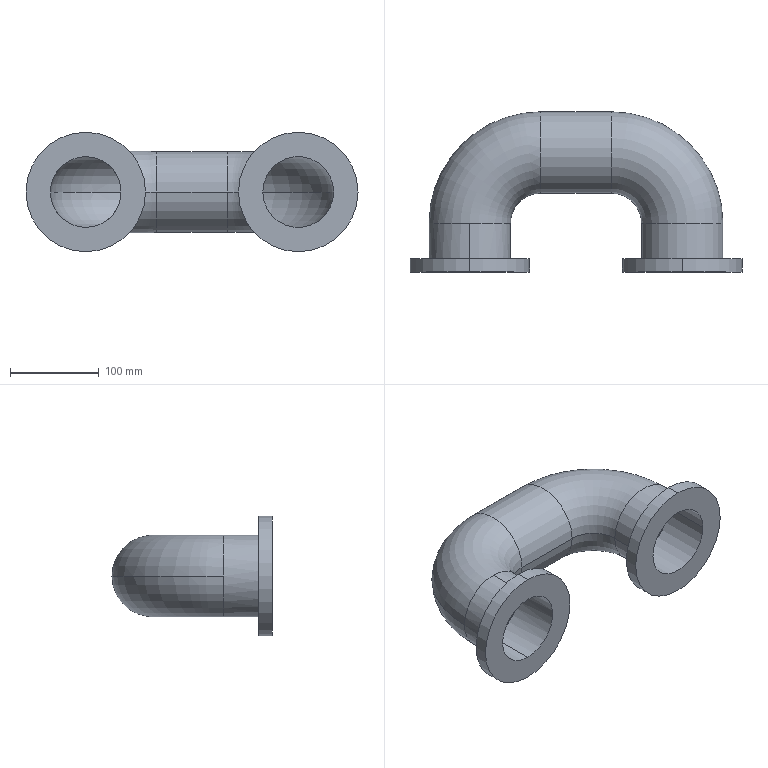Part | SolidWorks | features ICE 1, Sweep 1 | 1 solid | 28 faces | box 375 x 181 x 135 mm | volume 945407 mm3 | cylinder 16 | torus 8 | plane 4 | commonest cylinder face diameters 80 x6 92 x6 135 x4
STEP:
#1=CARTESIAN_POINT('',(160.,80.,0.));
#2=VERTEX_POINT('',#1);
#3=CARTESIAN_POINT('',(160.,160.,0.));
#4=VERTEX_POINT('',#3);
#5=CARTESIAN_POINT('',(160.,120.,0.));
#6=DIRECTION('',(-1.,0.,0.));
#7=DIRECTION('',(0.,0.,1.));
#8=AXIS2_PLACEMENT_3D('',#5,#6,#7);
#9=CIRCLE('',#8,40.);
#10=EDGE_CURVE('',#2,#4,#9,.T.);
#11=ORIENTED_EDGE('',*,*,#10,.T.);
#12=CARTESIAN_POINT('',(280.,40.,0.));
#13=VERTEX_POINT('',#12);
#14=CARTESIAN_POINT('',(160.,40.,0.));
#15=DIRECTION('',(0.,0.,-1.));
#16=DIRECTION('',(-1.,0.,0.));
#17=AXIS2_PLACEMENT_3D('',#14,#15,#16);
#18=CIRCLE('',#17,120.);
#19=EDGE_CURVE('',#4,#13,#18,.T.);
#20=ORIENTED_EDGE('',*,*,#19,.T.);
#21=CARTESIAN_POINT('',(200.,40.,0.));
#22=VERTEX_POINT('',#21);
#23=CARTESIAN_POINT('',(240.,40.,0.));
#24=DIRECTION('',(0.,1.,0.));
#25=DIRECTION('',(0.,0.,1.));
#26=AXIS2_PLACEMENT_3D('',#23,#24,#25);
#27=CIRCLE('',#26,40.);
#28=EDGE_CURVE('',#22,#13,#27,.T.);
#29=ORIENTED_EDGE('',*,*,#28,.F.);
#30=CARTESIAN_POINT('',(160.,40.,0.));
#31=DIRECTION('',(0.,0.,-1.));
#32=DIRECTION('',(-1.,0.,0.));
#33=AXIS2_PLACEMENT_3D('',#30,#31,#32);
#34=CIRCLE('',#33,40.);
#35=EDGE_CURVE('',#2,#22,#34,.T.);
#36=ORIENTED_EDGE('',*,*,#35,.F.);
#37=EDGE_LOOP('',(#11,#20,#29,#36));
#38=FACE_OUTER_BOUND('',#37,.T.);
#39=CARTESIAN_POINT('',(160.,40.,0.));
#40=DIRECTION('',(0.,0.,-1.));
#41=DIRECTION('',(-1.,0.,0.));
#42=AXIS2_PLACEMENT_3D('',#39,#40,#41);
#43=TOROIDAL_SURFACE('',#42,80.,40.);
#44=ADVANCED_FACE('',(#38),#43,.F.);
#45=CARTESIAN_POINT('',(0.,40.,40.));
#46=VERTEX_POINT('',#45);
#47=CARTESIAN_POINT('',(-40.,40.,0.));
#48=VERTEX_POINT('',#47);
#49=CARTESIAN_POINT('',(0.,40.,0.));
#50=DIRECTION('',(0.,-1.,0.));
#51=DIRECTION('',(0.,0.,1.));
#52=AXIS2_PLACEMENT_3D('',#49,#50,#51);
#53=CIRCLE('',#52,40.);
#54=EDGE_CURVE('',#46,#48,#53,.T.);
#55=ORIENTED_EDGE('',*,*,#54,.T.);
#56=CARTESIAN_POINT('',(80.,160.,0.));
#57=VERTEX_POINT('',#56);
#58=CARTESIAN_POINT('',(80.,40.,0.));
#59=DIRECTION('',(0.,0.,-1.));
#60=DIRECTION('',(-1.,0.,0.));
#61=AXIS2_PLACEMENT_3D('',#58,#59,#60);
#62=CIRCLE('',#61,120.);
#63=EDGE_CURVE('',#48,#57,#62,.T.);
#64=ORIENTED_EDGE('',*,*,#63,.T.);
#65=CARTESIAN_POINT('',(80.,80.,0.));
#66=VERTEX_POINT('',#65);
#67=CARTESIAN_POINT('',(80.,120.,0.));
#68=DIRECTION('',(-1.,0.,0.));
#69=DIRECTION('',(0.,0.,1.));
#70=AXIS2_PLACEMENT_3D('',#67,#68,#69);
#71=CIRCLE('',#70,40.);
#72=EDGE_CURVE('',#66,#57,#71,.T.);
#73=ORIENTED_EDGE('',*,*,#72,.F.);
#74=CARTESIAN_POINT('',(40.,40.,0.));
#75=VERTEX_POINT('',#74);
#76=CARTESIAN_POINT('',(80.,40.,0.));
#77=DIRECTION('',(0.,0.,-1.));
#78=DIRECTION('',(-1.,0.,0.));
#79=AXIS2_PLACEMENT_3D('',#76,#77,#78);
#80=CIRCLE('',#79,40.);
#81=EDGE_CURVE('',#75,#66,#80,.T.);
#82=ORIENTED_EDGE('',*,*,#81,.F.);
#83=CARTESIAN_POINT('',(0.,40.,0.));
#84=DIRECTION('',(0.,-1.,0.));
#85=DIRECTION('',(0.,0.,1.));
#86=AXIS2_PLACEMENT_3D('',#83,#84,#85);
#87=CIRCLE('',#86,40.);
#88=EDGE_CURVE('',#75,#46,#87,.T.);
#89=ORIENTED_EDGE('',*,*,#88,.T.);
#90=EDGE_LOOP('',(#55,#64,#73,#82,#89));
#91=FACE_OUTER_BOUND('',#90,.T.);
#92=CARTESIAN_POINT('',(80.,40.,0.));
#93=DIRECTION('',(0.,0.,-1.));
#94=DIRECTION('',(-1.,0.,0.));
#95=AXIS2_PLACEMENT_3D('',#92,#93,#94);
#96=TOROIDAL_SURFACE('',#95,80.,40.);
#97=ADVANCED_FACE('',(#91),#96,.F.);
#98=CARTESIAN_POINT('',(160.,74.,0.));
#99=VERTEX_POINT('',#98);
#100=CARTESIAN_POINT('',(160.,166.,0.));
#101=VERTEX_POINT('',#100);
#102=CARTESIAN_POINT('',(160.,120.,0.));
#103=DIRECTION('',(1.,0.,0.));
#104=DIRECTION('',(0.,0.,1.));
#105=AXIS2_PLACEMENT_3D('',#102,#103,#104);
#106=CIRCLE('',#105,46.);
#107=EDGE_CURVE('',#99,#101,#106,.T.);
#108=ORIENTED_EDGE('',*,*,#107,.T.);
#109=CARTESIAN_POINT('',(286.,40.,0.));
#110=VERTEX_POINT('',#109);
#111=CARTESIAN_POINT('',(160.,40.,0.));
#112=DIRECTION('',(0.,0.,-1.));
#113=DIRECTION('',(-1.,0.,0.));
#114=AXIS2_PLACEMENT_3D('',#111,#112,#113);
#115=CIRCLE('',#114,126.);
#116=EDGE_CURVE('',#101,#110,#115,.T.);
#117=ORIENTED_EDGE('',*,*,#116,.T.);
#118=CARTESIAN_POINT('',(194.,40.,0.));
#119=VERTEX_POINT('',#118);
#120=CARTESIAN_POINT('',(240.,40.,0.));
#121=DIRECTION('',(0.,-1.,0.));
#122=DIRECTION('',(0.,0.,1.));
#123=AXIS2_PLACEMENT_3D('',#120,#121,#122);
#124=CIRCLE('',#123,46.);
#125=EDGE_CURVE('',#119,#110,#124,.T.);
#126=ORIENTED_EDGE('',*,*,#125,.F.);
#127=CARTESIAN_POINT('',(160.,40.,0.));
#128=DIRECTION('',(0.,0.,-1.));
#129=DIRECTION('',(-1.,0.,0.));
#130=AXIS2_PLACEMENT_3D('',#127,#128,#129);
#131=CIRCLE('',#130,34.);
#132=EDGE_CURVE('',#99,#119,#131,.T.);
#133=ORIENTED_EDGE('',*,*,#132,.F.);
#134=EDGE_LOOP('',(#108,#117,#126,#133));
#135=FACE_OUTER_BOUND('',#134,.T.);
#136=CARTESIAN_POINT('',(160.,40.,0.));
#137=DIRECTION('',(0.,0.,-1.));
#138=DIRECTION('',(-1.,0.,0.));
#139=AXIS2_PLACEMENT_3D('',#136,#137,#138);
#140=TOROIDAL_SURFACE('',#139,80.,46.);
#141=ADVANCED_FACE('',(#135),#140,.T.);
#142=CARTESIAN_POINT('',(0.,40.,-46.));
#143=VERTEX_POINT('',#142);
#144=CARTESIAN_POINT('',(-46.,40.,0.));
#145=VERTEX_POINT('',#144);
#146=CARTESIAN_POINT('',(0.,40.,0.));
#147=DIRECTION('',(0.,1.,0.));
#148=DIRECTION('',(0.,0.,1.));
#149=AXIS2_PLACEMENT_3D('',#146,#147,#148);
#150=CIRCLE('',#149,46.);
#151=EDGE_CURVE('',#143,#145,#150,.T.);
#152=ORIENTED_EDGE('',*,*,#151,.T.);
#153=CARTESIAN_POINT('',(80.,166.,0.));
#154=VERTEX_POINT('',#153);
#155=CARTESIAN_POINT('',(80.,40.,0.));
#156=DIRECTION('',(0.,0.,-1.));
#157=DIRECTION('',(-1.,0.,0.));
#158=AXIS2_PLACEMENT_3D('',#155,#156,#157);
#159=CIRCLE('',#158,126.);
#160=EDGE_CURVE('',#145,#154,#159,.T.);
#161=ORIENTED_EDGE('',*,*,#160,.T.);
#162=CARTESIAN_POINT('',(80.,74.,0.));
#163=VERTEX_POINT('',#162);
#164=CARTESIAN_POINT('',(80.,120.,0.));
#165=DIRECTION('',(1.,0.,0.));
#166=DIRECTION('',(0.,0.,1.));
#167=AXIS2_PLACEMENT_3D('',#164,#165,#166);
#168=CIRCLE('',#167,46.);
#169=EDGE_CURVE('',#163,#154,#168,.T.);
#170=ORIENTED_EDGE('',*,*,#169,.F.);
#171=CARTESIAN_POINT('',(46.,40.,0.));
#172=VERTEX_POINT('',#171);
#173=CARTESIAN_POINT('',(80.,40.,0.));
#174=DIRECTION('',(0.,0.,-1.));
#175=DIRECTION('',(-1.,0.,0.));
#176=AXIS2_PLACEMENT_3D('',#173,#174,#175);
#177=CIRCLE('',#176,34.);
#178=EDGE_CURVE('',#172,#163,#177,.T.);
#179=ORIENTED_EDGE('',*,*,#178,.F.);
#180=CARTESIAN_POINT('',(0.,40.,0.));
#181=DIRECTION('',(0.,1.,0.));
#182=DIRECTION('',(0.,0.,1.));
#183=AXIS2_PLACEMENT_3D('',#180,#181,#182);
#184=CIRCLE('',#183,46.);
#185=EDGE_CURVE('',#172,#143,#184,.T.);
#186=ORIENTED_EDGE('',*,*,#185,.T.);
#187=EDGE_LOOP('',(#152,#161,#170,#179,#186));
#188=FACE_OUTER_BOUND('',#187,.T.);
#189=CARTESIAN_POINT('',(80.,40.,0.));
#190=DIRECTION('',(0.,0.,-1.));
#191=DIRECTION('',(-1.,0.,0.));
#192=AXIS2_PLACEMENT_3D('',#189,#190,#191);
#193=TOROIDAL_SURFACE('',#192,80.,46.);
#194=ADVANCED_FACE('',(#188),#193,.T.);
#195=CARTESIAN_POINT('',(240.,-15.,-67.5));
#196=VERTEX_POINT('',#195);
#197=CARTESIAN_POINT('',(240.,-15.,67.5));
#198=VERTEX_POINT('',#197);
#199=CARTESIAN_POINT('',(240.,-15.,0.));
#200=DIRECTION('',(0.,-1.,0.));
#201=DIRECTION('',(0.,0.,-1.));
#202=AXIS2_PLACEMENT_3D('',#199,#200,#201);
#203=CIRCLE('',#202,67.5);
#204=EDGE_CURVE('',#196,#198,#203,.T.);
#205=ORIENTED_EDGE('',*,*,#204,.F.);
#206=CARTESIAN_POINT('',(240.,0.,-67.5));
#207=VERTEX_POINT('',#206);
#208=CARTESIAN_POINT('',(240.,-15.,-67.5));
#209=DIRECTION('',(0.,1.,0.));
#210=VECTOR('',#209,1000.);
#211=LINE('',#208,#210);
#212=EDGE_CURVE('',#196,#207,#211,.T.);
#213=ORIENTED_EDGE('',*,*,#212,.T.);
#214=CARTESIAN_POINT('',(240.,0.,67.5));
#215=VERTEX_POINT('',#214);
#216=CARTESIAN_POINT('',(240.,0.,0.));
#217=DIRECTION('',(0.,-1.,0.));
#218=DIRECTION('',(0.,0.,-1.));
#219=AXIS2_PLACEMENT_3D('',#216,#217,#218);
#220=CIRCLE('',#219,67.5);
#221=EDGE_CURVE('',#207,#215,#220,.T.);
#222=ORIENTED_EDGE('',*,*,#221,.T.);
#223=CARTESIAN_POINT('',(240.,-15.,67.5));
#224=DIRECTION('',(0.,1.,0.));
#225=VECTOR('',#224,1000.);
#226=LINE('',#223,#225);
#227=EDGE_CURVE('',#198,#215,#226,.T.);
#228=ORIENTED_EDGE('',*,*,#227,.F.);
#229=EDGE_LOOP('',(#205,#213,#222,#228));
#230=FACE_OUTER_BOUND('',#229,.T.);
#231=CARTESIAN_POINT('',(240.,-15.,0.));
#232=DIRECTION('',(0.,1.,0.));
#233=DIRECTION('',(0.,0.,1.));
#234=AXIS2_PLACEMENT_3D('',#231,#232,#233);
#235=CYLINDRICAL_SURFACE('',#234,67.5);
#236=ADVANCED_FACE('',(#230),#235,.T.);
#237=CARTESIAN_POINT('',(0.,-15.,-67.5));
#238=VERTEX_POINT('',#237);
#239=CARTESIAN_POINT('',(0.,-15.,67.5));
#240=VERTEX_POINT('',#239);
#241=CARTESIAN_POINT('',(0.,-15.,0.));
#242=DIRECTION('',(0.,-1.,0.));
#243=DIRECTION('',(0.,0.,-1.));
#244=AXIS2_PLACEMENT_3D('',#241,#242,#243);
#245=CIRCLE('',#244,67.5);
#246=EDGE_CURVE('',#238,#240,#245,.T.);
#247=ORIENTED_EDGE('',*,*,#246,.F.);
#248=CARTESIAN_POINT('',(0.,0.,-67.5));
#249=VERTEX_POINT('',#248);
#250=CARTESIAN_POINT('',(0.,-15.,-67.5));
#251=DIRECTION('',(0.,1.,0.));
#252=VECTOR('',#251,1000.);
#253=LINE('',#250,#252);
#254=EDGE_CURVE('',#238,#249,#253,.T.);
#255=ORIENTED_EDGE('',*,*,#254,.T.);
#256=CARTESIAN_POINT('',(0.,0.,67.5));
#257=VERTEX_POINT('',#256);
#258=CARTESIAN_POINT('',(0.,0.,0.));
#259=DIRECTION('',(0.,-1.,0.));
#260=DIRECTION('',(0.,0.,-1.));
#261=AXIS2_PLACEMENT_3D('',#258,#259,#260);
#262=CIRCLE('',#261,67.5);
#263=EDGE_CURVE('',#249,#257,#262,.T.);
#264=ORIENTED_EDGE('',*,*,#263,.T.);
#265=CARTESIAN_POINT('',(0.,-15.,67.5));
#266=DIRECTION('',(0.,1.,0.));
#267=VECTOR('',#266,1000.);
#268=LINE('',#265,#267);
#269=EDGE_CURVE('',#240,#257,#268,.T.);
#270=ORIENTED_EDGE('',*,*,#269,.F.);
#271=EDGE_LOOP('',(#247,#255,#264,#270));
#272=FACE_OUTER_BOUND('',#271,.T.);
#273=CARTESIAN_POINT('',(0.,-15.,0.));
#274=DIRECTION('',(0.,1.,0.));
#275=DIRECTION('',(0.,0.,1.));
#276=AXIS2_PLACEMENT_3D('',#273,#274,#275);
#277=CYLINDRICAL_SURFACE('',#276,67.5);
#278=ADVANCED_FACE('',(#272),#277,.T.);
#279=CARTESIAN_POINT('',(240.,40.,0.));
#280=DIRECTION('',(0.,1.,0.));
#281=DIRECTION('',(0.,0.,1.));
#282=AXIS2_PLACEMENT_3D('',#279,#280,#281);
#283=CIRCLE('',#282,40.);
#284=EDGE_CURVE('',#13,#22,#283,.T.);
#285=ORIENTED_EDGE('',*,*,#284,.T.);
#286=CARTESIAN_POINT('',(200.,-15.,0.));
#287=VERTEX_POINT('',#286);
#288=CARTESIAN_POINT('',(200.,40.,0.));
#289=DIRECTION('',(0.,-1.,0.));
#290=VECTOR('',#289,1000.);
#291=LINE('',#288,#290);
#292=EDGE_CURVE('',#22,#287,#291,.T.);
#293=ORIENTED_EDGE('',*,*,#292,.T.);
#294=CARTESIAN_POINT('',(280.,-15.,0.));
#295=VERTEX_POINT('',#294);
#296=CARTESIAN_POINT('',(240.,-15.,0.));
#297=DIRECTION('',(0.,-1.,0.));
#298=DIRECTION('',(0.,0.,-1.));
#299=AXIS2_PLACEMENT_3D('',#296,#297,#298);
#300=CIRCLE('',#299,40.);
#301=EDGE_CURVE('',#287,#295,#300,.T.);
#302=ORIENTED_EDGE('',*,*,#301,.T.);
#303=CARTESIAN_POINT('',(280.,40.,0.));
#304=DIRECTION('',(0.,-1.,0.));
#305=VECTOR('',#304,1000.);
#306=LINE('',#303,#305);
#307=EDGE_CURVE('',#13,#295,#306,.T.);
#308=ORIENTED_EDGE('',*,*,#307,.F.);
#309=EDGE_LOOP('',(#285,#293,#302,#308));
#310=FACE_OUTER_BOUND('',#309,.T.);
#311=CARTESIAN_POINT('',(240.,40.,0.));
#312=DIRECTION('',(0.,-1.,0.));
#313=DIRECTION('',(1.,0.,0.));
#314=AXIS2_PLACEMENT_3D('',#311,#312,#313);
#315=CYLINDRICAL_SURFACE('',#314,40.);
#316=ADVANCED_FACE('',(#310),#315,.F.);
#317=CARTESIAN_POINT('',(80.,120.,0.));
#318=DIRECTION('',(-1.,0.,0.));
#319=DIRECTION('',(0.,0.,1.));
#320=AXIS2_PLACEMENT_3D('',#317,#318,#319);
#321=CIRCLE('',#320,40.);
#322=EDGE_CURVE('',#57,#66,#321,.T.);
#323=ORIENTED_EDGE('',*,*,#322,.T.);
#324=CARTESIAN_POINT('',(80.,80.,0.));
#325=DIRECTION('',(1.,0.,0.));
#326=VECTOR('',#325,1000.);
#327=LINE('',#324,#326);
#328=EDGE_CURVE('',#66,#2,#327,.T.);
#329=ORIENTED_EDGE('',*,*,#328,.T.);
#330=CARTESIAN_POINT('',(160.,120.,0.));
#331=DIRECTION('',(-1.,0.,0.));
#332=DIRECTION('',(0.,0.,1.));
#333=AXIS2_PLACEMENT_3D('',#330,#331,#332);
#334=CIRCLE('',#333,40.);
#335=EDGE_CURVE('',#4,#2,#334,.T.);
#336=ORIENTED_EDGE('',*,*,#335,.F.);
#337=CARTESIAN_POINT('',(80.,160.,0.));
#338=DIRECTION('',(1.,0.,0.));
#339=VECTOR('',#338,1000.);
#340=LINE('',#337,#339);
#341=EDGE_CURVE('',#57,#4,#340,.T.);
#342=ORIENTED_EDGE('',*,*,#341,.F.);
#343=EDGE_LOOP('',(#323,#329,#336,#342));
#344=FACE_OUTER_BOUND('',#343,.T.);
#345=CARTESIAN_POINT('',(80.,120.,0.));
#346=DIRECTION('',(1.,0.,0.));
#347=DIRECTION('',(0.,1.,0.));
#348=AXIS2_PLACEMENT_3D('',#345,#346,#347);
#349=CYLINDRICAL_SURFACE('',#348,40.);
#350=ADVANCED_FACE('',(#344),#349,.F.);
#351=CARTESIAN_POINT('',(0.,-15.,40.));
#352=VERTEX_POINT('',#351);
#353=CARTESIAN_POINT('',(0.,-15.,-40.));
#354=VERTEX_POINT('',#353);
#355=CARTESIAN_POINT('',(0.,-15.,0.));
#356=DIRECTION('',(0.,-1.,0.));
#357=DIRECTION('',(0.,0.,-1.));
#358=AXIS2_PLACEMENT_3D('',#355,#356,#357);
#359=CIRCLE('',#358,40.);
#360=EDGE_CURVE('',#352,#354,#359,.T.);
#361=ORIENTED_EDGE('',*,*,#360,.T.);
#362=CARTESIAN_POINT('',(0.,40.,-40.));
#363=VERTEX_POINT('',#362);
#364=CARTESIAN_POINT('',(0.,0.,-40.));
#365=DIRECTION('',(0.,1.,0.));
#366=VECTOR('',#365,1000.);
#367=LINE('',#364,#366);
#368=EDGE_CURVE('',#354,#363,#367,.T.);
#369=ORIENTED_EDGE('',*,*,#368,.T.);
#370=CARTESIAN_POINT('',(0.,40.,0.));
#371=DIRECTION('',(0.,-1.,0.));
#372=DIRECTION('',(0.,0.,1.));
#373=AXIS2_PLACEMENT_3D('',#370,#371,#372);
#374=CIRCLE('',#373,40.);
#375=EDGE_CURVE('',#48,#363,#374,.T.);
#376=ORIENTED_EDGE('',*,*,#375,.F.);
#377=ORIENTED_EDGE('',*,*,#54,.F.);
#378=CARTESIAN_POINT('',(0.,0.,40.));
#379=DIRECTION('',(0.,1.,0.));
#380=VECTOR('',#379,1000.);
#381=LINE('',#378,#380);
#382=EDGE_CURVE('',#352,#46,#381,.T.);
#383=ORIENTED_EDGE('',*,*,#382,.F.);
#384=EDGE_LOOP('',(#361,#369,#376,#377,#383));
#385=FACE_OUTER_BOUND('',#384,.T.);
#386=CARTESIAN_POINT('',(0.,0.,0.));
#387=DIRECTION('',(0.,1.,0.));
#388=DIRECTION('',(0.,0.,1.));
#389=AXIS2_PLACEMENT_3D('',#386,#387,#388);
#390=CYLINDRICAL_SURFACE('',#389,40.);
#391=ADVANCED_FACE('',(#385),#390,.F.);
#392=CARTESIAN_POINT('',(240.,40.,0.));
#393=DIRECTION('',(0.,-1.,0.));
#394=DIRECTION('',(0.,0.,1.));
#395=AXIS2_PLACEMENT_3D('',#392,#393,#394);
#396=CIRCLE('',#395,46.);
#397=EDGE_CURVE('',#110,#119,#396,.T.);
#398=ORIENTED_EDGE('',*,*,#397,.T.);
#399=CARTESIAN_POINT('',(194.,0.,0.));
#400=VERTEX_POINT('',#399);
#401=CARTESIAN_POINT('',(194.,40.,0.));
#402=DIRECTION('',(0.,-1.,0.));
#403=VECTOR('',#402,1000.);
#404=LINE('',#401,#403);
#405=EDGE_CURVE('',#119,#400,#404,.T.);
#406=ORIENTED_EDGE('',*,*,#405,.T.);
#407=CARTESIAN_POINT('',(286.,0.,0.));
#408=VERTEX_POINT('',#407);
#409=CARTESIAN_POINT('',(240.,0.,0.));
#410=DIRECTION('',(0.,-1.,0.));
#411=DIRECTION('',(0.,0.,1.));
#412=AXIS2_PLACEMENT_3D('',#409,#410,#411);
#413=CIRCLE('',#412,46.);
#414=EDGE_CURVE('',#408,#400,#413,.T.);
#415=ORIENTED_EDGE('',*,*,#414,.F.);
#416=CARTESIAN_POINT('',(286.,40.,0.));
#417=DIRECTION('',(0.,-1.,0.));
#418=VECTOR('',#417,1000.);
#419=LINE('',#416,#418);
#420=EDGE_CURVE('',#110,#408,#419,.T.);
#421=ORIENTED_EDGE('',*,*,#420,.F.);
#422=EDGE_LOOP('',(#398,#406,#415,#421));
#423=FACE_OUTER_BOUND('',#422,.T.);
#424=CARTESIAN_POINT('',(240.,40.,0.));
#425=DIRECTION('',(0.,-1.,0.));
#426=DIRECTION('',(1.,0.,0.));
#427=AXIS2_PLACEMENT_3D('',#424,#425,#426);
#428=CYLINDRICAL_SURFACE('',#427,46.);
#429=ADVANCED_FACE('',(#423),#428,.T.);
#430=CARTESIAN_POINT('',(80.,120.,0.));
#431=DIRECTION('',(1.,0.,0.));
#432=DIRECTION('',(0.,0.,1.));
#433=AXIS2_PLACEMENT_3D('',#430,#431,#432);
#434=CIRCLE('',#433,46.);
#435=EDGE_CURVE('',#154,#163,#434,.T.);
#436=ORIENTED_EDGE('',*,*,#435,.T.);
#437=CARTESIAN_POINT('',(80.,74.,0.));
#438=DIRECTION('',(1.,0.,0.));
#439=VECTOR('',#438,1000.);
#440=LINE('',#437,#439);
#441=EDGE_CURVE('',#163,#99,#440,.T.);
#442=ORIENTED_EDGE('',*,*,#441,.T.);
#443=CARTESIAN_POINT('',(160.,120.,0.));
#444=DIRECTION('',(1.,0.,0.));
#445=DIRECTION('',(0.,0.,1.));
#446=AXIS2_PLACEMENT_3D('',#443,#444,#445);
#447=CIRCLE('',#446,46.);
#448=EDGE_CURVE('',#101,#99,#447,.T.);
#449=ORIENTED_EDGE('',*,*,#448,.F.);
#450=CARTESIAN_POINT('',(80.,166.,0.));
#451=DIRECTION('',(1.,0.,0.));
#452=VECTOR('',#451,1000.);
#453=LINE('',#450,#452);
#454=EDGE_CURVE('',#154,#101,#453,.T.);
#455=ORIENTED_EDGE('',*,*,#454,.F.);
#456=EDGE_LOOP('',(#436,#442,#449,#455));
#457=FACE_OUTER_BOUND('',#456,.T.);
#458=CARTESIAN_POINT('',(80.,120.,0.));
#459=DIRECTION('',(1.,0.,0.));
#460=DIRECTION('',(0.,1.,0.));
#461=AXIS2_PLACEMENT_3D('',#458,#459,#460);
#462=CYLINDRICAL_SURFACE('',#461,46.);
#463=ADVANCED_FACE('',(#457),#462,.T.);
#464=CARTESIAN_POINT('',(0.,0.,46.));
#465=VERTEX_POINT('',#464);
#466=CARTESIAN_POINT('',(0.,0.,-46.));
#467=VERTEX_POINT('',#466);
#468=CARTESIAN_POINT('',(0.,0.,0.));
#469=DIRECTION('',(0.,1.,0.));
#470=DIRECTION('',(0.,0.,1.));
#471=AXIS2_PLACEMENT_3D('',#468,#469,#470);
#472=CIRCLE('',#471,46.);
#473=EDGE_CURVE('',#465,#467,#472,.T.);
#474=ORIENTED_EDGE('',*,*,#473,.T.);
#475=CARTESIAN_POINT('',(0.,0.,-46.));
#476=DIRECTION('',(0.,1.,0.));
#477=VECTOR('',#476,1000.);
#478=LINE('',#475,#477);
#479=EDGE_CURVE('',#467,#143,#478,.T.);
#480=ORIENTED_EDGE('',*,*,#479,.T.);
#481=ORIENTED_EDGE('',*,*,#185,.F.);
#482=CARTESIAN_POINT('',(0.,40.,46.));
#483=VERTEX_POINT('',#482);
#484=CARTESIAN_POINT('',(0.,40.,0.));
#485=DIRECTION('',(0.,1.,0.));
#486=DIRECTION('',(0.,0.,1.));
#487=AXIS2_PLACEMENT_3D('',#484,#485,#486);
#488=CIRCLE('',#487,46.);
#489=EDGE_CURVE('',#483,#172,#488,.T.);
#490=ORIENTED_EDGE('',*,*,#489,.F.);
#491=CARTESIAN_POINT('',(0.,0.,46.));
#492=DIRECTION('',(0.,1.,0.));
#493=VECTOR('',#492,1000.);
#494=LINE('',#491,#493);
#495=EDGE_CURVE('',#465,#483,#494,.T.);
#496=ORIENTED_EDGE('',*,*,#495,.F.);
#497=EDGE_LOOP('',(#474,#480,#481,#490,#496));
#498=FACE_OUTER_BOUND('',#497,.T.);
#499=CARTESIAN_POINT('',(0.,0.,0.));
#500=DIRECTION('',(0.,1.,0.));
#501=DIRECTION('',(0.,0.,1.));
#502=AXIS2_PLACEMENT_3D('',#499,#500,#501);
#503=CYLINDRICAL_SURFACE('',#502,46.);
#504=ADVANCED_FACE('',(#498),#503,.T.);
#505=ORIENTED_EDGE('',*,*,#292,.F.);
#506=ORIENTED_EDGE('',*,*,#28,.T.);
#507=ORIENTED_EDGE('',*,*,#307,.T.);
#508=CARTESIAN_POINT('',(240.,-15.,0.));
#509=DIRECTION('',(0.,-1.,0.));
#510=DIRECTION('',(0.,0.,-1.));
#511=AXIS2_PLACEMENT_3D('',#508,#509,#510);
#512=CIRCLE('',#511,40.);
#513=EDGE_CURVE('',#295,#287,#512,.T.);
#514=ORIENTED_EDGE('',*,*,#513,.T.);
#515=EDGE_LOOP('',(#505,#506,#507,#514));
#516=FACE_OUTER_BOUND('',#515,.T.);
#517=CARTESIAN_POINT('',(240.,40.,0.));
#518=DIRECTION('',(0.,-1.,0.));
#519=DIRECTION('',(1.,0.,0.));
#520=AXIS2_PLACEMENT_3D('',#517,#518,#519);
#521=CYLINDRICAL_SURFACE('',#520,40.);
#522=ADVANCED_FACE('',(#516),#521,.F.);
#523=ORIENTED_EDGE('',*,*,#19,.F.);
#524=ORIENTED_EDGE('',*,*,#335,.T.);
#525=ORIENTED_EDGE('',*,*,#35,.T.);
#526=ORIENTED_EDGE('',*,*,#284,.F.);
#527=EDGE_LOOP('',(#523,#524,#525,#526));
#528=FACE_OUTER_BOUND('',#527,.T.);
#529=CARTESIAN_POINT('',(160.,40.,0.));
#530=DIRECTION('',(0.,0.,-1.));
#531=DIRECTION('',(-1.,0.,0.));
#532=AXIS2_PLACEMENT_3D('',#529,#530,#531);
#533=TOROIDAL_SURFACE('',#532,80.,40.);
#534=ADVANCED_FACE('',(#528),#533,.F.);
#535=ORIENTED_EDGE('',*,*,#328,.F.);
#536=ORIENTED_EDGE('',*,*,#72,.T.);
#537=ORIENTED_EDGE('',*,*,#341,.T.);
#538=ORIENTED_EDGE('',*,*,#10,.F.);
#539=EDGE_LOOP('',(#535,#536,#537,#538));
#540=FACE_OUTER_BOUND('',#539,.T.);
#541=CARTESIAN_POINT('',(80.,120.,0.));
#542=DIRECTION('',(1.,0.,0.));
#543=DIRECTION('',(0.,1.,0.));
#544=AXIS2_PLACEMENT_3D('',#541,#542,#543);
#545=CYLINDRICAL_SURFACE('',#544,40.);
#546=ADVANCED_FACE('',(#540),#545,.F.);
#547=ORIENTED_EDGE('',*,*,#63,.F.);
#548=ORIENTED_EDGE('',*,*,#375,.T.);
#549=CARTESIAN_POINT('',(0.,40.,0.));
#550=DIRECTION('',(0.,-1.,0.));
#551=DIRECTION('',(0.,0.,1.));
#552=AXIS2_PLACEMENT_3D('',#549,#550,#551);
#553=CIRCLE('',#552,40.);
#554=EDGE_CURVE('',#363,#75,#553,.T.);
#555=ORIENTED_EDGE('',*,*,#554,.T.);
#556=ORIENTED_EDGE('',*,*,#81,.T.);
#557=ORIENTED_EDGE('',*,*,#322,.F.);
#558=EDGE_LOOP('',(#547,#548,#555,#556,#557));
#559=FACE_OUTER_BOUND('',#558,.T.);
#560=CARTESIAN_POINT('',(80.,40.,0.));
#561=DIRECTION('',(0.,0.,-1.));
#562=DIRECTION('',(-1.,0.,0.));
#563=AXIS2_PLACEMENT_3D('',#560,#561,#562);
#564=TOROIDAL_SURFACE('',#563,80.,40.);
#565=ADVANCED_FACE('',(#559),#564,.F.);
#566=ORIENTED_EDGE('',*,*,#368,.F.);
#567=CARTESIAN_POINT('',(0.,-15.,0.));
#568=DIRECTION('',(0.,-1.,0.));
#569=DIRECTION('',(0.,0.,-1.));
#570=AXIS2_PLACEMENT_3D('',#567,#568,#569);
#571=CIRCLE('',#570,40.);
#572=EDGE_CURVE('',#354,#352,#571,.T.);
#573=ORIENTED_EDGE('',*,*,#572,.T.);
#574=ORIENTED_EDGE('',*,*,#382,.T.);
#575=ORIENTED_EDGE('',*,*,#88,.F.);
#576=ORIENTED_EDGE('',*,*,#554,.F.);
#577=EDGE_LOOP('',(#566,#573,#574,#575,#576));
#578=FACE_OUTER_BOUND('',#577,.T.);
#579=CARTESIAN_POINT('',(0.,0.,0.));
#580=DIRECTION('',(0.,1.,0.));
#581=DIRECTION('',(0.,0.,1.));
#582=AXIS2_PLACEMENT_3D('',#579,#580,#581);
#583=CYLINDRICAL_SURFACE('',#582,40.);
#584=ADVANCED_FACE('',(#578),#583,.F.);
#585=ORIENTED_EDGE('',*,*,#405,.F.);
#586=ORIENTED_EDGE('',*,*,#125,.T.);
#587=ORIENTED_EDGE('',*,*,#420,.T.);
#588=CARTESIAN_POINT('',(240.,0.,0.));
#589=DIRECTION('',(0.,-1.,0.));
#590=DIRECTION('',(0.,0.,1.));
#591=AXIS2_PLACEMENT_3D('',#588,#589,#590);
#592=CIRCLE('',#591,46.);
#593=EDGE_CURVE('',#400,#408,#592,.T.);
#594=ORIENTED_EDGE('',*,*,#593,.F.);
#595=EDGE_LOOP('',(#585,#586,#587,#594));
#596=FACE_OUTER_BOUND('',#595,.T.);
#597=CARTESIAN_POINT('',(240.,40.,0.));
#598=DIRECTION('',(0.,-1.,0.));
#599=DIRECTION('',(1.,0.,0.));
#600=AXIS2_PLACEMENT_3D('',#597,#598,#599);
#601=CYLINDRICAL_SURFACE('',#600,46.);
#602=ADVANCED_FACE('',(#596),#601,.T.);
#603=ORIENTED_EDGE('',*,*,#116,.F.);
#604=ORIENTED_EDGE('',*,*,#448,.T.);
#605=ORIENTED_EDGE('',*,*,#132,.T.);
#606=ORIENTED_EDGE('',*,*,#397,.F.);
#607=EDGE_LOOP('',(#603,#604,#605,#606));
#608=FACE_OUTER_BOUND('',#607,.T.);
#609=CARTESIAN_POINT('',(160.,40.,0.));
#610=DIRECTION('',(0.,0.,-1.));
#611=DIRECTION('',(-1.,0.,0.));
#612=AXIS2_PLACEMENT_3D('',#609,#610,#611);
#613=TOROIDAL_SURFACE('',#612,80.,46.);
#614=ADVANCED_FACE('',(#608),#613,.T.);
#615=ORIENTED_EDGE('',*,*,#441,.F.);
#616=ORIENTED_EDGE('',*,*,#169,.T.);
#617=ORIENTED_EDGE('',*,*,#454,.T.);
#618=ORIENTED_EDGE('',*,*,#107,.F.);
#619=EDGE_LOOP('',(#615,#616,#617,#618));
#620=FACE_OUTER_BOUND('',#619,.T.);
#621=CARTESIAN_POINT('',(80.,120.,0.));
#622=DIRECTION('',(1.,0.,0.));
#623=DIRECTION('',(0.,1.,0.));
#624=AXIS2_PLACEMENT_3D('',#621,#622,#623);
#625=CYLINDRICAL_SURFACE('',#624,46.);
#626=ADVANCED_FACE('',(#620),#625,.T.);
#627=ORIENTED_EDGE('',*,*,#160,.F.);
#628=CARTESIAN_POINT('',(0.,40.,0.));
#629=DIRECTION('',(0.,1.,0.));
#630=DIRECTION('',(0.,0.,1.));
#631=AXIS2_PLACEMENT_3D('',#628,#629,#630);
#632=CIRCLE('',#631,46.);
#633=EDGE_CURVE('',#145,#483,#632,.T.);
#634=ORIENTED_EDGE('',*,*,#633,.T.);
#635=ORIENTED_EDGE('',*,*,#489,.T.);
#636=ORIENTED_EDGE('',*,*,#178,.T.);
#637=ORIENTED_EDGE('',*,*,#435,.F.);
#638=EDGE_LOOP('',(#627,#634,#635,#636,#637));
#639=FACE_OUTER_BOUND('',#638,.T.);
#640=CARTESIAN_POINT('',(80.,40.,0.));
#641=DIRECTION('',(0.,0.,-1.));
#642=DIRECTION('',(-1.,0.,0.));
#643=AXIS2_PLACEMENT_3D('',#640,#641,#642);
#644=TOROIDAL_SURFACE('',#643,80.,46.);
#645=ADVANCED_FACE('',(#639),#644,.T.);
#646=ORIENTED_EDGE('',*,*,#479,.F.);
#647=CARTESIAN_POINT('',(0.,0.,0.));
#648=DIRECTION('',(0.,1.,0.));
#649=DIRECTION('',(0.,0.,1.));
#650=AXIS2_PLACEMENT_3D('',#647,#648,#649);
#651=CIRCLE('',#650,46.);
#652=EDGE_CURVE('',#467,#465,#651,.T.);
#653=ORIENTED_EDGE('',*,*,#652,.T.);
#654=ORIENTED_EDGE('',*,*,#495,.T.);
#655=ORIENTED_EDGE('',*,*,#633,.F.);
#656=ORIENTED_EDGE('',*,*,#151,.F.);
#657=EDGE_LOOP('',(#646,#653,#654,#655,#656));
#658=FACE_OUTER_BOUND('',#657,.T.);
#659=CARTESIAN_POINT('',(0.,0.,0.));
#660=DIRECTION('',(0.,1.,0.));
#661=DIRECTION('',(0.,0.,1.));
#662=AXIS2_PLACEMENT_3D('',#659,#660,#661);
#663=CYLINDRICAL_SURFACE('',#662,46.);
#664=ADVANCED_FACE('',(#658),#663,.T.);
#665=CARTESIAN_POINT('',(0.,-15.,0.));
#666=DIRECTION('',(0.,-1.,0.));
#667=DIRECTION('',(0.,0.,-1.));
#668=AXIS2_PLACEMENT_3D('',#665,#666,#667);
#669=CIRCLE('',#668,67.5);
#670=EDGE_CURVE('',#240,#238,#669,.T.);
#671=ORIENTED_EDGE('',*,*,#670,.T.);
#672=ORIENTED_EDGE('',*,*,#246,.T.);
#673=EDGE_LOOP('',(#671,#672));
#674=FACE_OUTER_BOUND('',#673,.T.);
#675=ORIENTED_EDGE('',*,*,#360,.F.);
#676=ORIENTED_EDGE('',*,*,#572,.F.);
#677=EDGE_LOOP('',(#675,#676));
#678=FACE_BOUND('',#677,.T.);
#679=CARTESIAN_POINT('',(0.,-15.,0.));
#680=DIRECTION('',(0.,-1.,0.));
#681=DIRECTION('',(0.,0.,-1.));
#682=AXIS2_PLACEMENT_3D('',#679,#680,#681);
#683=PLANE('',#682);
#684=ADVANCED_FACE('',(#674,#678),#683,.T.);
#685=ORIENTED_EDGE('',*,*,#473,.F.);
#686=ORIENTED_EDGE('',*,*,#652,.F.);
#687=EDGE_LOOP('',(#685,#686));
#688=FACE_BOUND('',#687,.T.);
#689=CARTESIAN_POINT('',(0.,0.,0.));
#690=DIRECTION('',(0.,-1.,0.));
#691=DIRECTION('',(0.,0.,-1.));
#692=AXIS2_PLACEMENT_3D('',#689,#690,#691);
#693=CIRCLE('',#692,67.5);
#694=EDGE_CURVE('',#257,#249,#693,.T.);
#695=ORIENTED_EDGE('',*,*,#694,.F.);
#696=ORIENTED_EDGE('',*,*,#263,.F.);
#697=EDGE_LOOP('',(#695,#696));
#698=FACE_OUTER_BOUND('',#697,.T.);
#699=CARTESIAN_POINT('',(0.,0.,0.));
#700=DIRECTION('',(0.,-1.,0.));
#701=DIRECTION('',(0.,0.,-1.));
#702=AXIS2_PLACEMENT_3D('',#699,#700,#701);
#703=PLANE('',#702);
#704=ADVANCED_FACE('',(#688,#698),#703,.F.);
#705=ORIENTED_EDGE('',*,*,#254,.F.);
#706=ORIENTED_EDGE('',*,*,#670,.F.);
#707=ORIENTED_EDGE('',*,*,#269,.T.);
#708=ORIENTED_EDGE('',*,*,#694,.T.);
#709=EDGE_LOOP('',(#705,#706,#707,#708));
#710=FACE_OUTER_BOUND('',#709,.T.);
#711=CARTESIAN_POINT('',(0.,-15.,0.));
#712=DIRECTION('',(0.,1.,0.));
#713=DIRECTION('',(0.,0.,1.));
#714=AXIS2_PLACEMENT_3D('',#711,#712,#713);
#715=CYLINDRICAL_SURFACE('',#714,67.5);
#716=ADVANCED_FACE('',(#710),#715,.T.);
#717=CARTESIAN_POINT('',(240.,-15.,0.));
#718=DIRECTION('',(0.,-1.,0.));
#719=DIRECTION('',(0.,0.,-1.));
#720=AXIS2_PLACEMENT_3D('',#717,#718,#719);
#721=CIRCLE('',#720,67.5);
#722=EDGE_CURVE('',#198,#196,#721,.T.);
#723=ORIENTED_EDGE('',*,*,#722,.T.);
#724=ORIENTED_EDGE('',*,*,#204,.T.);
#725=EDGE_LOOP('',(#723,#724));
#726=FACE_OUTER_BOUND('',#725,.T.);
#727=ORIENTED_EDGE('',*,*,#513,.F.);
#728=ORIENTED_EDGE('',*,*,#301,.F.);
#729=EDGE_LOOP('',(#727,#728));
#730=FACE_BOUND('',#729,.T.);
#731=CARTESIAN_POINT('',(240.,-15.,0.));
#732=DIRECTION('',(0.,-1.,0.));
#733=DIRECTION('',(0.,0.,-1.));
#734=AXIS2_PLACEMENT_3D('',#731,#732,#733);
#735=PLANE('',#734);
#736=ADVANCED_FACE('',(#726,#730),#735,.T.);
#737=ORIENTED_EDGE('',*,*,#414,.T.);
#738=ORIENTED_EDGE('',*,*,#593,.T.);
#739=EDGE_LOOP('',(#737,#738));
#740=FACE_BOUND('',#739,.T.);
#741=CARTESIAN_POINT('',(240.,0.,0.));
#742=DIRECTION('',(0.,-1.,0.));
#743=DIRECTION('',(0.,0.,-1.));
#744=AXIS2_PLACEMENT_3D('',#741,#742,#743);
#745=CIRCLE('',#744,67.5);
#746=EDGE_CURVE('',#215,#207,#745,.T.);
#747=ORIENTED_EDGE('',*,*,#746,.F.);
#748=ORIENTED_EDGE('',*,*,#221,.F.);
#749=EDGE_LOOP('',(#747,#748));
#750=FACE_OUTER_BOUND('',#749,.T.);
#751=CARTESIAN_POINT('',(240.,0.,0.));
#752=DIRECTION('',(0.,-1.,0.));
#753=DIRECTION('',(0.,0.,-1.));
#754=AXIS2_PLACEMENT_3D('',#751,#752,#753);
#755=PLANE('',#754);
#756=ADVANCED_FACE('',(#740,#750),#755,.F.);
#757=ORIENTED_EDGE('',*,*,#212,.F.);
#758=ORIENTED_EDGE('',*,*,#722,.F.);
#759=ORIENTED_EDGE('',*,*,#227,.T.);
#760=ORIENTED_EDGE('',*,*,#746,.T.);
#761=EDGE_LOOP('',(#757,#758,#759,#760));
#762=FACE_OUTER_BOUND('',#761,.T.);
#763=CARTESIAN_POINT('',(240.,-15.,0.));
#764=DIRECTION('',(0.,1.,0.));
#765=DIRECTION('',(0.,0.,1.));
#766=AXIS2_PLACEMENT_3D('',#763,#764,#765);
#767=CYLINDRICAL_SURFACE('',#766,67.5);
#768=ADVANCED_FACE('',(#762),#767,.T.);
#769=CLOSED_SHELL('',(#44,#97,#141,#194,#236,#278,#316,#350,#391,#429,#463,#504,#522,#534,#546,#565,#584,#602,#614,#626,#645,#664,#684,#704,#716,#736,#756,#768));
#770=MANIFOLD_SOLID_BREP('',#769);
#771=CARTESIAN_POINT('',(0.,0.,0.));
#772=DIRECTION('',(0.,0.,1.));
#773=DIRECTION('',(1.,0.,0.));
#774=AXIS2_PLACEMENT_3D('',#771,#772,#773);
#775=(LENGTH_UNIT()NAMED_UNIT(*)SI_UNIT(.MILLI.,.METRE.));
#776=UNCERTAINTY_MEASURE_WITH_UNIT(LENGTH_MEASURE(0.00001),#775,'','');
#777=(NAMED_UNIT(*)PLANE_ANGLE_UNIT()SI_UNIT($,.RADIAN.));
#778=(NAMED_UNIT(*)SI_UNIT($,.STERADIAN.)SOLID_ANGLE_UNIT());
#779=(GEOMETRIC_REPRESENTATION_CONTEXT(3)GLOBAL_UNCERTAINTY_ASSIGNED_CONTEXT((#776))GLOBAL_UNIT_ASSIGNED_CONTEXT((#775,#777,#778))REPRESENTATION_CONTEXT('',''));
#780=ADVANCED_BREP_SHAPE_REPRESENTATION('',(#770,#774),#779);